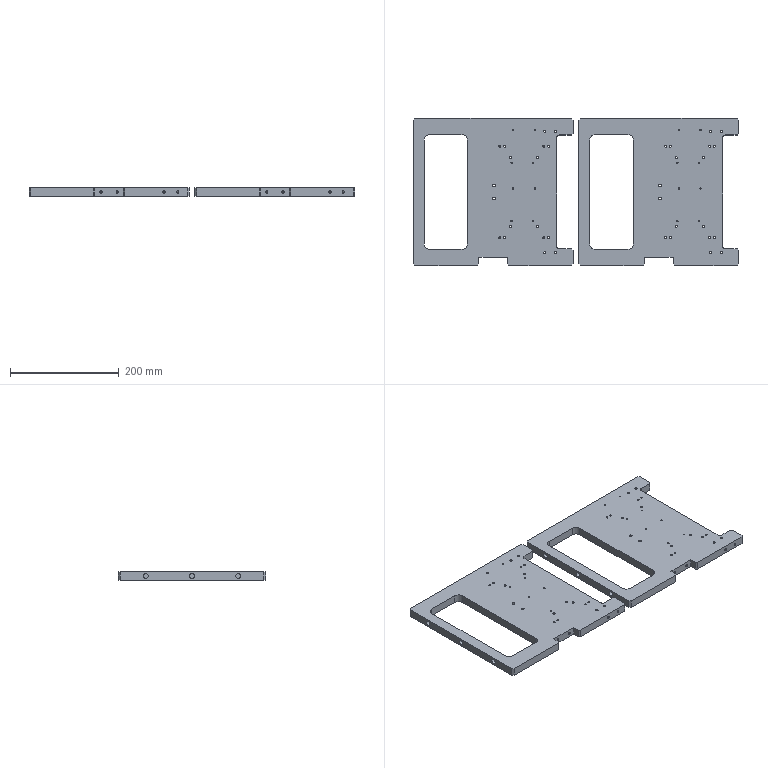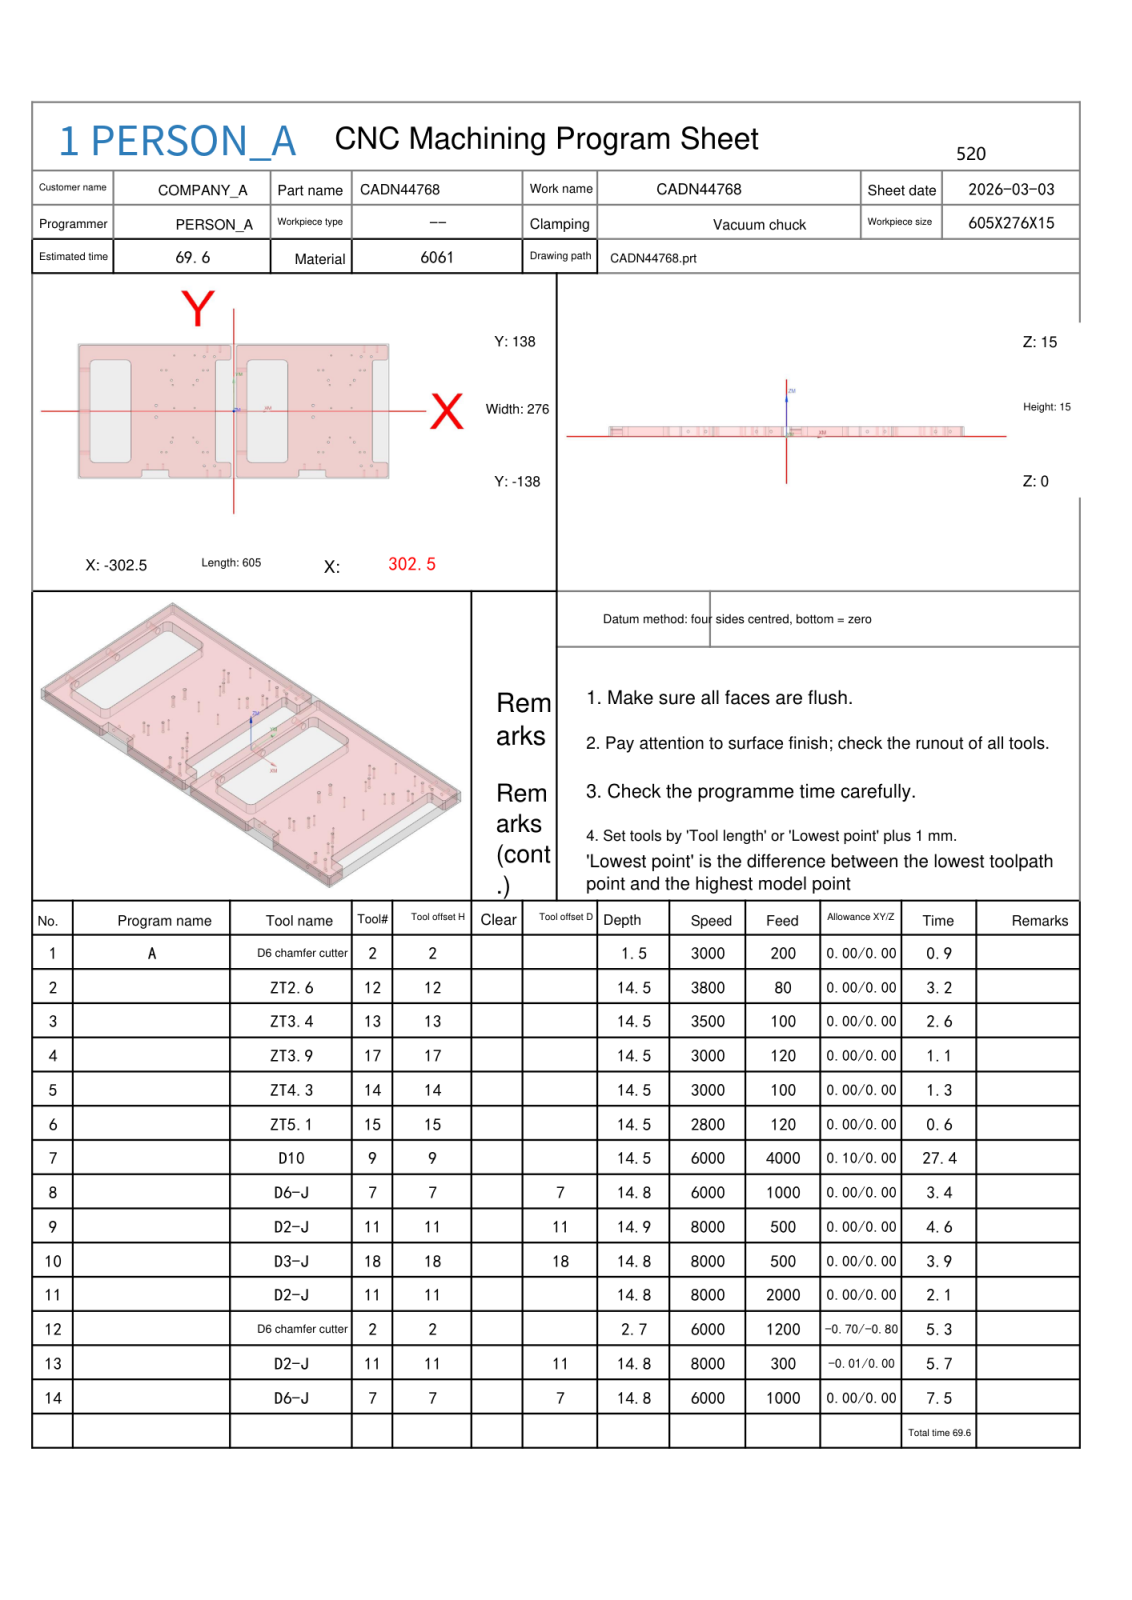NC program | NX | posted by the shop | part box 600 x 271 x 15 mm
Lines 3033 to 3155 of 17346:
N8 T07 M06
(D6-J  D=6. R=0. H=07 ce=0.00 di=0.00)
(D.N=07 MAX_Z=45. MIN_Z=0.2 Time=3.43M)
G00 G90 G54 X101.216 Y-96.5 M03 S6000
G43 H07 Z45.
M08
Z8.25
G01 Z7.75 F1000.
G41 D07
X101.5
G03 X102.5 Y-95.5 I0.0 J1.
G01 Y95.5
G03 X95.5 Y102.5 I-7. J0.0
G01 X35.5
G03 X28.5 Y95.5 I0.0 J-7.
G01 Y-95.5
G03 X35.5 Y-102.5 I7. J0.0
G01 X95.5
G03 X102.5 Y-95.5 I0.0 J7.
G01 Y-95.
G03 X101.5 Y-94. I-1. J0.0
G01 G40 X101.3
Z8.25
G00 X101.216 Y-96.5
Z1.
G01 Z.5
G41 D07
X101.5
G03 X102.5 Y-95.5 I0.0 J1.
G01 Y95.5
G03 X95.5 Y102.5 I-7. J0.0
G01 X35.5
G03 X28.5 Y95.5 I0.0 J-7.
G01 Y-95.5
G03 X35.5 Y-102.5 I7. J0.0
G01 X95.5
G03 X102.5 Y-95.5 I0.0 J7.
G01 Y-95.
G03 X101.5 Y-94. I-1. J0.0
G01 G40 X101.3
Z1.
G00 Z45.
X-275.716 Y96.5
Z8.25
G01 Z7.75
G41 D07
X-276.
G03 X-277. Y95.5 I0.0 J-1.
G01 Y-95.5
G03 X-270. Y-102.5 I7. J0.0
G01 X-210.
G03 X-203. Y-95.5 I0.0 J7.
G01 Y95.5
G03 X-210. Y102.5 I-7. J0.0
G01 X-270.
G03 X-277. Y95.5 I0.0 J-7.
G01 Y95.
G03 X-276. Y94. I1. J0.0
G01 G40 X-275.8
Z8.25
G00 X-275.716 Y96.5
Z1.
G01 Z.5
G41 D07
X-276.
G03 X-277. Y95.5 I0.0 J-1.
G01 Y-95.5
G03 X-270. Y-102.5 I7. J0.0
G01 X-210.
G03 X-203. Y-95.5 I0.0 J7.
G01 Y95.5
G03 X-210. Y102.5 I-7. J0.0
G01 X-270.
G03 X-277. Y95.5 I0.0 J-7.
G01 Y95.
G03 X-276. Y94. I1. J0.0
G01 G40 X-275.8
Z1.
G00 Z45.
G00 G90 X101.316 Y-96.5 M03 S6000
Z45.
Z.7
G01 Z.2 F1000.
G41 D07
X101.5
G03 X102.5 Y-95.5 I0.0 J1.
G01 Y95.5
G03 X95.5 Y102.5 I-7. J0.0
G01 X35.5
G03 X28.5 Y95.5 I0.0 J-7.
G01 Y-95.5
G03 X35.5 Y-102.5 I7. J0.0
G01 X95.5
G03 X102.5 Y-95.5 I0.0 J7.
G01 Y-95.
G03 X101.5 Y-94. I-1. J0.0
G01 G40 X101.4
Z.7
G00 Z45.
X-275.816 Y96.5
Z.7
G01 Z.2
G41 D07
X-276.
G03 X-277. Y95.5 I0.0 J-1.
G01 Y-95.5
G03 X-270. Y-102.5 I7. J0.0
G01 X-210.
G03 X-203. Y-95.5 I0.0 J7.
G01 Y95.5
G03 X-210. Y102.5 I-7. J0.0
G01 X-270.
G03 X-277. Y95.5 I0.0 J-7.
G01 Y95.
G03 X-276. Y94. I1. J0.0
G01 G40 X-275.9
Z.7
G00 Z45.
G91 G28 Z0.0
M05
M09
G91 G28 Z0.0
M01